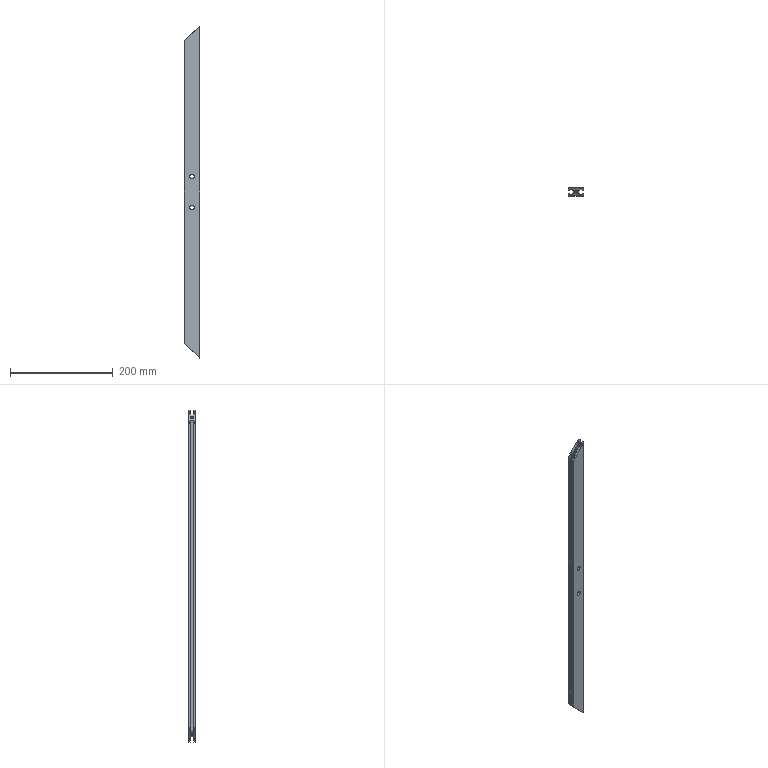Part | NX | features BREP 1 | 1 solid | 127 faces | box 30 x 15 x 647 mm | volume 147250 mm3 | cylinder 65 | plane 54 | cone 8 | commonest cylinder face diameters 5 x23 1 x18 3.3 x16 2 x4 8.5 x4